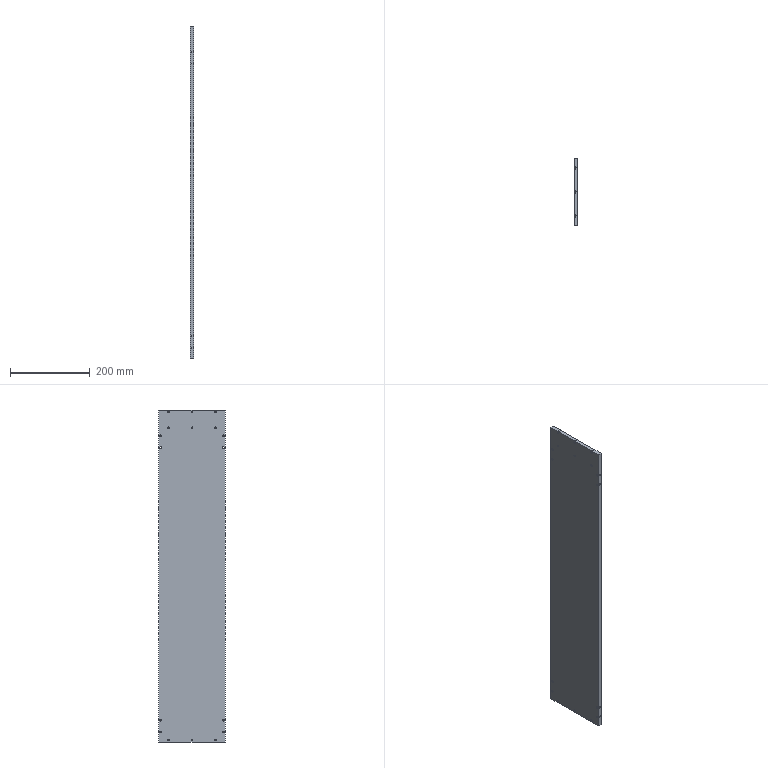Part | STEP file | 03-25 Support cross plate | 1 solid | 91 faces | box 10 x 168 x 835 mm | volume 1395635 mm3 | cylinder 68 | plane 23 | commonest cylinder face diameters 4.5 x34 9 x34